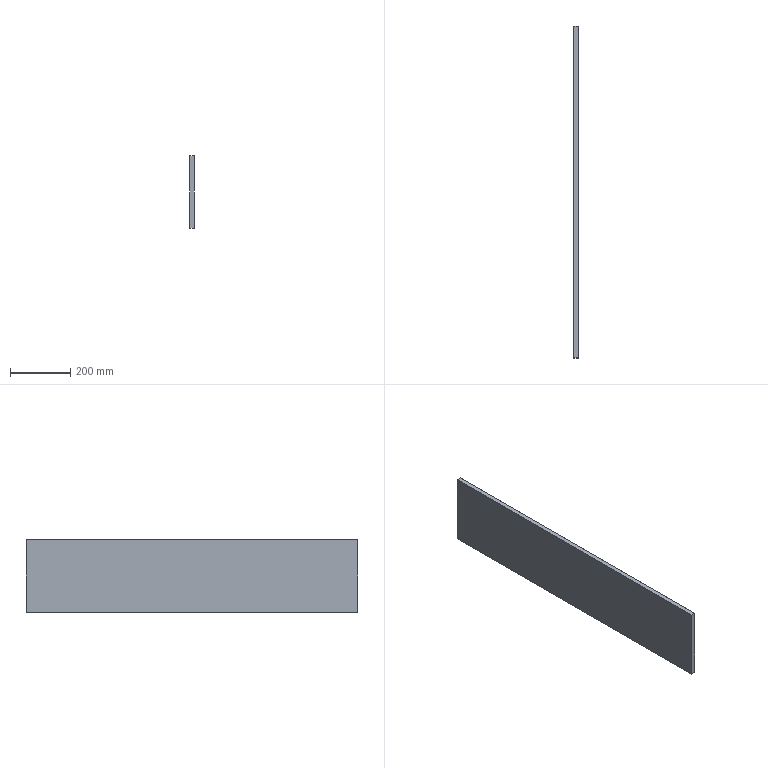Part | STEP file | HJDX-203 | 1 solid | 26 faces | box 16 x 1100 x 240 mm | volume 4223323 mm3 | plane 26
STEP:
#1=CARTESIAN_POINT('',(16.,-549.5,-119.5));
#2=VERTEX_POINT('',#1);
#3=CARTESIAN_POINT('',(16.,-549.5,119.5));
#4=VERTEX_POINT('',#3);
#5=CARTESIAN_POINT('',(16.,-549.5,0.));
#6=DIRECTION('',(0.,0.,1.));
#7=VECTOR('',#6,1000.);
#8=LINE('',#5,#7);
#9=EDGE_CURVE('',#2,#4,#8,.T.);
#10=ORIENTED_EDGE('',*,*,#9,.F.);
#11=CARTESIAN_POINT('',(16.,549.5,-119.5));
#12=VERTEX_POINT('',#11);
#13=CARTESIAN_POINT('',(16.,0.,-119.5));
#14=DIRECTION('',(0.,-1.,0.));
#15=VECTOR('',#14,1000.);
#16=LINE('',#13,#15);
#17=EDGE_CURVE('',#12,#2,#16,.T.);
#18=ORIENTED_EDGE('',*,*,#17,.F.);
#19=CARTESIAN_POINT('',(16.,549.5,119.5));
#20=VERTEX_POINT('',#19);
#21=CARTESIAN_POINT('',(16.,549.5,0.));
#22=DIRECTION('',(0.,0.,-1.));
#23=VECTOR('',#22,1000.);
#24=LINE('',#21,#23);
#25=EDGE_CURVE('',#20,#12,#24,.T.);
#26=ORIENTED_EDGE('',*,*,#25,.F.);
#27=CARTESIAN_POINT('',(16.,0.,119.5));
#28=DIRECTION('',(0.,1.,0.));
#29=VECTOR('',#28,1000.);
#30=LINE('',#27,#29);
#31=EDGE_CURVE('',#4,#20,#30,.T.);
#32=ORIENTED_EDGE('',*,*,#31,.F.);
#33=EDGE_LOOP('',(#10,#18,#26,#32));
#34=FACE_OUTER_BOUND('',#33,.T.);
#35=CARTESIAN_POINT('',(16.,0.,0.));
#36=DIRECTION('',(-1.,0.,0.));
#37=DIRECTION('',(0.,0.,1.));
#38=AXIS2_PLACEMENT_3D('',#35,#36,#37);
#39=PLANE('',#38);
#40=ADVANCED_FACE('',(#34),#39,.F.);
#41=CARTESIAN_POINT('',(15.5,-549.5,120.));
#42=VERTEX_POINT('',#41);
#43=CARTESIAN_POINT('',(15.5,549.5,120.));
#44=VERTEX_POINT('',#43);
#45=CARTESIAN_POINT('',(15.5,0.,120.));
#46=DIRECTION('',(0.,1.,0.));
#47=VECTOR('',#46,1000.);
#48=LINE('',#45,#47);
#49=EDGE_CURVE('',#42,#44,#48,.T.);
#50=ORIENTED_EDGE('',*,*,#49,.F.);
#51=CARTESIAN_POINT('',(16.,-549.5,119.5));
#52=DIRECTION('',(-0.7071,0.,0.7071));
#53=VECTOR('',#52,1000.);
#54=LINE('',#51,#53);
#55=EDGE_CURVE('',#4,#42,#54,.T.);
#56=ORIENTED_EDGE('',*,*,#55,.F.);
#57=ORIENTED_EDGE('',*,*,#31,.T.);
#58=CARTESIAN_POINT('',(16.,549.5,119.5));
#59=DIRECTION('',(0.7071,0.,-0.7071));
#60=VECTOR('',#59,1000.);
#61=LINE('',#58,#60);
#62=EDGE_CURVE('',#44,#20,#61,.T.);
#63=ORIENTED_EDGE('',*,*,#62,.F.);
#64=EDGE_LOOP('',(#50,#56,#57,#63));
#65=FACE_OUTER_BOUND('',#64,.T.);
#66=CARTESIAN_POINT('',(16.,0.,119.5));
#67=DIRECTION('',(-0.7071,0.,-0.7071));
#68=DIRECTION('',(-0.7071,0.,0.7071));
#69=AXIS2_PLACEMENT_3D('',#66,#67,#68);
#70=PLANE('',#69);
#71=ADVANCED_FACE('',(#65),#70,.F.);
#72=CARTESIAN_POINT('',(15.5,-550.,-119.5));
#73=VERTEX_POINT('',#72);
#74=CARTESIAN_POINT('',(15.5,-550.,119.5));
#75=VERTEX_POINT('',#74);
#76=CARTESIAN_POINT('',(15.5,-550.,0.));
#77=DIRECTION('',(0.,0.,1.));
#78=VECTOR('',#77,1000.);
#79=LINE('',#76,#78);
#80=EDGE_CURVE('',#73,#75,#79,.T.);
#81=ORIENTED_EDGE('',*,*,#80,.F.);
#82=CARTESIAN_POINT('',(16.,-549.5,-119.5));
#83=DIRECTION('',(-0.7071,-0.7071,0.));
#84=VECTOR('',#83,1000.);
#85=LINE('',#82,#84);
#86=EDGE_CURVE('',#2,#73,#85,.T.);
#87=ORIENTED_EDGE('',*,*,#86,.F.);
#88=ORIENTED_EDGE('',*,*,#9,.T.);
#89=CARTESIAN_POINT('',(16.,-549.5,119.5));
#90=DIRECTION('',(0.7071,0.7071,0.));
#91=VECTOR('',#90,1000.);
#92=LINE('',#89,#91);
#93=EDGE_CURVE('',#75,#4,#92,.T.);
#94=ORIENTED_EDGE('',*,*,#93,.F.);
#95=EDGE_LOOP('',(#81,#87,#88,#94));
#96=FACE_OUTER_BOUND('',#95,.T.);
#97=CARTESIAN_POINT('',(16.,-549.5,0.));
#98=DIRECTION('',(-0.7071,0.7071,0.));
#99=DIRECTION('',(-0.7071,-0.7071,0.));
#100=AXIS2_PLACEMENT_3D('',#97,#98,#99);
#101=PLANE('',#100);
#102=ADVANCED_FACE('',(#96),#101,.F.);
#103=ORIENTED_EDGE('',*,*,#17,.T.);
#104=CARTESIAN_POINT('',(15.5,-549.5,-120.));
#105=VERTEX_POINT('',#104);
#106=CARTESIAN_POINT('',(16.,-549.5,-119.5));
#107=DIRECTION('',(0.7071,0.,0.7071));
#108=VECTOR('',#107,1000.);
#109=LINE('',#106,#108);
#110=EDGE_CURVE('',#105,#2,#109,.T.);
#111=ORIENTED_EDGE('',*,*,#110,.F.);
#112=CARTESIAN_POINT('',(15.5,549.5,-120.));
#113=VERTEX_POINT('',#112);
#114=CARTESIAN_POINT('',(15.5,0.,-120.));
#115=DIRECTION('',(0.,-1.,0.));
#116=VECTOR('',#115,1000.);
#117=LINE('',#114,#116);
#118=EDGE_CURVE('',#113,#105,#117,.T.);
#119=ORIENTED_EDGE('',*,*,#118,.F.);
#120=CARTESIAN_POINT('',(16.,549.5,-119.5));
#121=DIRECTION('',(-0.7071,0.,-0.7071));
#122=VECTOR('',#121,1000.);
#123=LINE('',#120,#122);
#124=EDGE_CURVE('',#12,#113,#123,.T.);
#125=ORIENTED_EDGE('',*,*,#124,.F.);
#126=EDGE_LOOP('',(#103,#111,#119,#125));
#127=FACE_OUTER_BOUND('',#126,.T.);
#128=CARTESIAN_POINT('',(16.,0.,-119.5));
#129=DIRECTION('',(-0.7071,0.,0.7071));
#130=DIRECTION('',(0.7071,0.,0.7071));
#131=AXIS2_PLACEMENT_3D('',#128,#129,#130);
#132=PLANE('',#131);
#133=ADVANCED_FACE('',(#127),#132,.F.);
#134=ORIENTED_EDGE('',*,*,#25,.T.);
#135=CARTESIAN_POINT('',(15.5,550.,-119.5));
#136=VERTEX_POINT('',#135);
#137=CARTESIAN_POINT('',(16.,549.5,-119.5));
#138=DIRECTION('',(0.7071,-0.7071,0.));
#139=VECTOR('',#138,1000.);
#140=LINE('',#137,#139);
#141=EDGE_CURVE('',#136,#12,#140,.T.);
#142=ORIENTED_EDGE('',*,*,#141,.F.);
#143=CARTESIAN_POINT('',(15.5,550.,119.5));
#144=VERTEX_POINT('',#143);
#145=CARTESIAN_POINT('',(15.5,550.,0.));
#146=DIRECTION('',(0.,0.,-1.));
#147=VECTOR('',#146,1000.);
#148=LINE('',#145,#147);
#149=EDGE_CURVE('',#144,#136,#148,.T.);
#150=ORIENTED_EDGE('',*,*,#149,.F.);
#151=CARTESIAN_POINT('',(16.,549.5,119.5));
#152=DIRECTION('',(-0.7071,0.7071,0.));
#153=VECTOR('',#152,1000.);
#154=LINE('',#151,#153);
#155=EDGE_CURVE('',#20,#144,#154,.T.);
#156=ORIENTED_EDGE('',*,*,#155,.F.);
#157=EDGE_LOOP('',(#134,#142,#150,#156));
#158=FACE_OUTER_BOUND('',#157,.T.);
#159=CARTESIAN_POINT('',(16.,549.5,0.));
#160=DIRECTION('',(-0.7071,-0.7071,0.));
#161=DIRECTION('',(0.7071,-0.7071,0.));
#162=AXIS2_PLACEMENT_3D('',#159,#160,#161);
#163=PLANE('',#162);
#164=ADVANCED_FACE('',(#158),#163,.F.);
#165=CARTESIAN_POINT('',(15.5,549.5,120.));
#166=DIRECTION('',(0.,-0.7071,0.7071));
#167=VECTOR('',#166,1000.);
#168=LINE('',#165,#167);
#169=EDGE_CURVE('',#144,#44,#168,.T.);
#170=ORIENTED_EDGE('',*,*,#169,.T.);
#171=ORIENTED_EDGE('',*,*,#62,.T.);
#172=ORIENTED_EDGE('',*,*,#155,.T.);
#173=EDGE_LOOP('',(#170,#171,#172));
#174=FACE_OUTER_BOUND('',#173,.T.);
#175=CARTESIAN_POINT('',(15.5,550.,119.5));
#176=DIRECTION('',(0.5774,0.5774,0.5774));
#177=DIRECTION('',(0.7071,0.,-0.7071));
#178=AXIS2_PLACEMENT_3D('',#175,#176,#177);
#179=PLANE('',#178);
#180=ADVANCED_FACE('',(#174),#179,.T.);
#181=CARTESIAN_POINT('',(0.5,549.5,120.));
#182=VERTEX_POINT('',#181);
#183=CARTESIAN_POINT('',(16.,549.5,120.));
#184=DIRECTION('',(1.,0.,0.));
#185=VECTOR('',#184,1000.);
#186=LINE('',#183,#185);
#187=EDGE_CURVE('',#182,#44,#186,.T.);
#188=ORIENTED_EDGE('',*,*,#187,.F.);
#189=CARTESIAN_POINT('',(0.5,-549.5,120.));
#190=VERTEX_POINT('',#189);
#191=CARTESIAN_POINT('',(0.5,-550.,120.));
#192=DIRECTION('',(0.,1.,0.));
#193=VECTOR('',#192,1000.);
#194=LINE('',#191,#193);
#195=EDGE_CURVE('',#190,#182,#194,.T.);
#196=ORIENTED_EDGE('',*,*,#195,.F.);
#197=CARTESIAN_POINT('',(16.,-549.5,120.));
#198=DIRECTION('',(-1.,0.,0.));
#199=VECTOR('',#198,1000.);
#200=LINE('',#197,#199);
#201=EDGE_CURVE('',#42,#190,#200,.T.);
#202=ORIENTED_EDGE('',*,*,#201,.F.);
#203=ORIENTED_EDGE('',*,*,#49,.T.);
#204=EDGE_LOOP('',(#188,#196,#202,#203));
#205=FACE_OUTER_BOUND('',#204,.T.);
#206=CARTESIAN_POINT('',(16.,-550.,120.));
#207=DIRECTION('',(0.,0.,-1.));
#208=DIRECTION('',(-1.,0.,0.));
#209=AXIS2_PLACEMENT_3D('',#206,#207,#208);
#210=PLANE('',#209);
#211=ADVANCED_FACE('',(#205),#210,.F.);
#212=CARTESIAN_POINT('',(15.5,-549.5,120.));
#213=DIRECTION('',(0.,-0.7071,-0.7071));
#214=VECTOR('',#213,1000.);
#215=LINE('',#212,#214);
#216=EDGE_CURVE('',#42,#75,#215,.T.);
#217=ORIENTED_EDGE('',*,*,#216,.T.);
#218=ORIENTED_EDGE('',*,*,#93,.T.);
#219=ORIENTED_EDGE('',*,*,#55,.T.);
#220=EDGE_LOOP('',(#217,#218,#219));
#221=FACE_OUTER_BOUND('',#220,.T.);
#222=CARTESIAN_POINT('',(15.5,-549.5,120.));
#223=DIRECTION('',(0.5774,-0.5774,0.5774));
#224=DIRECTION('',(0.7071,0.,-0.7071));
#225=AXIS2_PLACEMENT_3D('',#222,#223,#224);
#226=PLANE('',#225);
#227=ADVANCED_FACE('',(#221),#226,.T.);
#228=CARTESIAN_POINT('',(0.5,-550.,-119.5));
#229=VERTEX_POINT('',#228);
#230=CARTESIAN_POINT('',(16.,-550.,-119.5));
#231=DIRECTION('',(-1.,0.,0.));
#232=VECTOR('',#231,1000.);
#233=LINE('',#230,#232);
#234=EDGE_CURVE('',#73,#229,#233,.T.);
#235=ORIENTED_EDGE('',*,*,#234,.F.);
#236=ORIENTED_EDGE('',*,*,#80,.T.);
#237=CARTESIAN_POINT('',(0.5,-550.,119.5));
#238=VERTEX_POINT('',#237);
#239=CARTESIAN_POINT('',(16.,-550.,119.5));
#240=DIRECTION('',(1.,0.,0.));
#241=VECTOR('',#240,1000.);
#242=LINE('',#239,#241);
#243=EDGE_CURVE('',#238,#75,#242,.T.);
#244=ORIENTED_EDGE('',*,*,#243,.F.);
#245=CARTESIAN_POINT('',(0.5,-550.,120.));
#246=DIRECTION('',(0.,0.,1.));
#247=VECTOR('',#246,1000.);
#248=LINE('',#245,#247);
#249=EDGE_CURVE('',#229,#238,#248,.T.);
#250=ORIENTED_EDGE('',*,*,#249,.F.);
#251=EDGE_LOOP('',(#235,#236,#244,#250));
#252=FACE_OUTER_BOUND('',#251,.T.);
#253=CARTESIAN_POINT('',(16.,-550.,120.));
#254=DIRECTION('',(0.,1.,0.));
#255=DIRECTION('',(0.,0.,1.));
#256=AXIS2_PLACEMENT_3D('',#253,#254,#255);
#257=PLANE('',#256);
#258=ADVANCED_FACE('',(#252),#257,.F.);
#259=ORIENTED_EDGE('',*,*,#86,.T.);
#260=CARTESIAN_POINT('',(15.5,-550.,-119.5));
#261=DIRECTION('',(0.,0.7071,-0.7071));
#262=VECTOR('',#261,1000.);
#263=LINE('',#260,#262);
#264=EDGE_CURVE('',#73,#105,#263,.T.);
#265=ORIENTED_EDGE('',*,*,#264,.T.);
#266=ORIENTED_EDGE('',*,*,#110,.T.);
#267=EDGE_LOOP('',(#259,#265,#266));
#268=FACE_OUTER_BOUND('',#267,.T.);
#269=CARTESIAN_POINT('',(15.5,-550.,-119.5));
#270=DIRECTION('',(0.5774,-0.5774,-0.5774));
#271=DIRECTION('',(-0.7071,0.,-0.7071));
#272=AXIS2_PLACEMENT_3D('',#269,#270,#271);
#273=PLANE('',#272);
#274=ADVANCED_FACE('',(#268),#273,.T.);
#275=ORIENTED_EDGE('',*,*,#141,.T.);
#276=ORIENTED_EDGE('',*,*,#124,.T.);
#277=CARTESIAN_POINT('',(15.5,550.,-119.5));
#278=DIRECTION('',(0.,0.7071,0.7071));
#279=VECTOR('',#278,1000.);
#280=LINE('',#277,#279);
#281=EDGE_CURVE('',#113,#136,#280,.T.);
#282=ORIENTED_EDGE('',*,*,#281,.T.);
#283=EDGE_LOOP('',(#275,#276,#282));
#284=FACE_OUTER_BOUND('',#283,.T.);
#285=CARTESIAN_POINT('',(15.5,549.5,-120.));
#286=DIRECTION('',(0.5774,0.5774,-0.5774));
#287=DIRECTION('',(-0.7071,0.,-0.7071));
#288=AXIS2_PLACEMENT_3D('',#285,#286,#287);
#289=PLANE('',#288);
#290=ADVANCED_FACE('',(#284),#289,.T.);
#291=CARTESIAN_POINT('',(0.5,549.5,-120.));
#292=VERTEX_POINT('',#291);
#293=CARTESIAN_POINT('',(0.5,-549.5,-120.));
#294=VERTEX_POINT('',#293);
#295=CARTESIAN_POINT('',(0.5,-550.,-120.));
#296=DIRECTION('',(0.,-1.,0.));
#297=VECTOR('',#296,1000.);
#298=LINE('',#295,#297);
#299=EDGE_CURVE('',#292,#294,#298,.T.);
#300=ORIENTED_EDGE('',*,*,#299,.F.);
#301=CARTESIAN_POINT('',(16.,549.5,-120.));
#302=DIRECTION('',(-1.,0.,0.));
#303=VECTOR('',#302,1000.);
#304=LINE('',#301,#303);
#305=EDGE_CURVE('',#113,#292,#304,.T.);
#306=ORIENTED_EDGE('',*,*,#305,.F.);
#307=ORIENTED_EDGE('',*,*,#118,.T.);
#308=CARTESIAN_POINT('',(16.,-549.5,-120.));
#309=DIRECTION('',(1.,0.,0.));
#310=VECTOR('',#309,1000.);
#311=LINE('',#308,#310);
#312=EDGE_CURVE('',#294,#105,#311,.T.);
#313=ORIENTED_EDGE('',*,*,#312,.F.);
#314=EDGE_LOOP('',(#300,#306,#307,#313));
#315=FACE_OUTER_BOUND('',#314,.T.);
#316=CARTESIAN_POINT('',(16.,-550.,-120.));
#317=DIRECTION('',(0.,0.,1.));
#318=DIRECTION('',(1.,0.,0.));
#319=AXIS2_PLACEMENT_3D('',#316,#317,#318);
#320=PLANE('',#319);
#321=ADVANCED_FACE('',(#315),#320,.F.);
#322=CARTESIAN_POINT('',(0.5,550.,119.5));
#323=VERTEX_POINT('',#322);
#324=CARTESIAN_POINT('',(0.5,550.,-119.5));
#325=VERTEX_POINT('',#324);
#326=CARTESIAN_POINT('',(0.5,550.,120.));
#327=DIRECTION('',(0.,0.,-1.));
#328=VECTOR('',#327,1000.);
#329=LINE('',#326,#328);
#330=EDGE_CURVE('',#323,#325,#329,.T.);
#331=ORIENTED_EDGE('',*,*,#330,.F.);
#332=CARTESIAN_POINT('',(16.,550.,119.5));
#333=DIRECTION('',(-1.,0.,0.));
#334=VECTOR('',#333,1000.);
#335=LINE('',#332,#334);
#336=EDGE_CURVE('',#144,#323,#335,.T.);
#337=ORIENTED_EDGE('',*,*,#336,.F.);
#338=ORIENTED_EDGE('',*,*,#149,.T.);
#339=CARTESIAN_POINT('',(16.,550.,-119.5));
#340=DIRECTION('',(1.,0.,0.));
#341=VECTOR('',#340,1000.);
#342=LINE('',#339,#341);
#343=EDGE_CURVE('',#325,#136,#342,.T.);
#344=ORIENTED_EDGE('',*,*,#343,.F.);
#345=EDGE_LOOP('',(#331,#337,#338,#344));
#346=FACE_OUTER_BOUND('',#345,.T.);
#347=CARTESIAN_POINT('',(16.,550.,120.));
#348=DIRECTION('',(0.,-1.,0.));
#349=DIRECTION('',(0.,0.,-1.));
#350=AXIS2_PLACEMENT_3D('',#347,#348,#349);
#351=PLANE('',#350);
#352=ADVANCED_FACE('',(#346),#351,.F.);
#353=ORIENTED_EDGE('',*,*,#336,.T.);
#354=CARTESIAN_POINT('',(0.5,549.5,120.));
#355=DIRECTION('',(0.,0.7071,-0.7071));
#356=VECTOR('',#355,1000.);
#357=LINE('',#354,#356);
#358=EDGE_CURVE('',#182,#323,#357,.T.);
#359=ORIENTED_EDGE('',*,*,#358,.F.);
#360=ORIENTED_EDGE('',*,*,#187,.T.);
#361=ORIENTED_EDGE('',*,*,#169,.F.);
#362=EDGE_LOOP('',(#353,#359,#360,#361));
#363=FACE_OUTER_BOUND('',#362,.T.);
#364=CARTESIAN_POINT('',(16.,549.5,120.));
#365=DIRECTION('',(0.,-0.7071,-0.7071));
#366=DIRECTION('',(0.,0.7071,-0.7071));
#367=AXIS2_PLACEMENT_3D('',#364,#365,#366);
#368=PLANE('',#367);
#369=ADVANCED_FACE('',(#363),#368,.F.);
#370=CARTESIAN_POINT('',(0.,-549.5,119.5));
#371=VERTEX_POINT('',#370);
#372=CARTESIAN_POINT('',(0.5,-549.5,120.));
#373=DIRECTION('',(0.7071,0.,0.7071));
#374=VECTOR('',#373,1000.);
#375=LINE('',#372,#374);
#376=EDGE_CURVE('',#371,#190,#375,.T.);
#377=ORIENTED_EDGE('',*,*,#376,.T.);
#378=ORIENTED_EDGE('',*,*,#195,.T.);
#379=CARTESIAN_POINT('',(0.,549.5,119.5));
#380=VERTEX_POINT('',#379);
#381=CARTESIAN_POINT('',(0.5,549.5,120.));
#382=DIRECTION('',(-0.7071,0.,-0.7071));
#383=VECTOR('',#382,1000.);
#384=LINE('',#381,#383);
#385=EDGE_CURVE('',#182,#380,#384,.T.);
#386=ORIENTED_EDGE('',*,*,#385,.T.);
#387=CARTESIAN_POINT('',(0.,-550.,119.5));
#388=DIRECTION('',(0.,-1.,0.));
#389=VECTOR('',#388,1000.);
#390=LINE('',#387,#389);
#391=EDGE_CURVE('',#380,#371,#390,.T.);
#392=ORIENTED_EDGE('',*,*,#391,.T.);
#393=EDGE_LOOP('',(#377,#378,#386,#392));
#394=FACE_OUTER_BOUND('',#393,.T.);
#395=CARTESIAN_POINT('',(0.5,-550.,120.));
#396=DIRECTION('',(-0.7071,0.,0.7071));
#397=DIRECTION('',(0.7071,0.,0.7071));
#398=AXIS2_PLACEMENT_3D('',#395,#396,#397);
#399=PLANE('',#398);
#400=ADVANCED_FACE('',(#394),#399,.T.);
#401=ORIENTED_EDGE('',*,*,#201,.T.);
#402=CARTESIAN_POINT('',(0.5,-550.,119.5));
#403=DIRECTION('',(0.,0.7071,0.7071));
#404=VECTOR('',#403,1000.);
#405=LINE('',#402,#404);
#406=EDGE_CURVE('',#238,#190,#405,.T.);
#407=ORIENTED_EDGE('',*,*,#406,.F.);
#408=ORIENTED_EDGE('',*,*,#243,.T.);
#409=ORIENTED_EDGE('',*,*,#216,.F.);
#410=EDGE_LOOP('',(#401,#407,#408,#409));
#411=FACE_OUTER_BOUND('',#410,.T.);
#412=CARTESIAN_POINT('',(16.,-550.,119.5));
#413=DIRECTION('',(0.,0.7071,-0.7071));
#414=DIRECTION('',(0.,0.7071,0.7071));
#415=AXIS2_PLACEMENT_3D('',#412,#413,#414);
#416=PLANE('',#415);
#417=ADVANCED_FACE('',(#411),#416,.F.);
#418=CARTESIAN_POINT('',(0.,-549.5,-119.5));
#419=VERTEX_POINT('',#418);
#420=CARTESIAN_POINT('',(0.5,-550.,-119.5));
#421=DIRECTION('',(0.7071,-0.7071,0.));
#422=VECTOR('',#421,1000.);
#423=LINE('',#420,#422);
#424=EDGE_CURVE('',#419,#229,#423,.T.);
#425=ORIENTED_EDGE('',*,*,#424,.T.);
#426=ORIENTED_EDGE('',*,*,#249,.T.);
#427=CARTESIAN_POINT('',(0.5,-550.,119.5));
#428=DIRECTION('',(-0.7071,0.7071,0.));
#429=VECTOR('',#428,1000.);
#430=LINE('',#427,#429);
#431=EDGE_CURVE('',#238,#371,#430,.T.);
#432=ORIENTED_EDGE('',*,*,#431,.T.);
#433=CARTESIAN_POINT('',(0.,-549.5,120.));
#434=DIRECTION('',(0.,0.,-1.));
#435=VECTOR('',#434,1000.);
#436=LINE('',#433,#435);
#437=EDGE_CURVE('',#371,#419,#436,.T.);
#438=ORIENTED_EDGE('',*,*,#437,.T.);
#439=EDGE_LOOP('',(#425,#426,#432,#438));
#440=FACE_OUTER_BOUND('',#439,.T.);
#441=CARTESIAN_POINT('',(0.5,-550.,120.));
#442=DIRECTION('',(-0.7071,-0.7071,0.));
#443=DIRECTION('',(0.7071,-0.7071,0.));
#444=AXIS2_PLACEMENT_3D('',#441,#442,#443);
#445=PLANE('',#444);
#446=ADVANCED_FACE('',(#440),#445,.T.);
#447=ORIENTED_EDGE('',*,*,#234,.T.);
#448=CARTESIAN_POINT('',(0.5,-549.5,-120.));
#449=DIRECTION('',(0.,-0.7071,0.7071));
#450=VECTOR('',#449,1000.);
#451=LINE('',#448,#450);
#452=EDGE_CURVE('',#294,#229,#451,.T.);
#453=ORIENTED_EDGE('',*,*,#452,.F.);
#454=ORIENTED_EDGE('',*,*,#312,.T.);
#455=ORIENTED_EDGE('',*,*,#264,.F.);
#456=EDGE_LOOP('',(#447,#453,#454,#455));
#457=FACE_OUTER_BOUND('',#456,.T.);
#458=CARTESIAN_POINT('',(16.,-549.5,-120.));
#459=DIRECTION('',(0.,0.7071,0.7071));
#460=DIRECTION('',(0.,-0.7071,0.7071));
#461=AXIS2_PLACEMENT_3D('',#458,#459,#460);
#462=PLANE('',#461);
#463=ADVANCED_FACE('',(#457),#462,.F.);
#464=CARTESIAN_POINT('',(0.5,-549.5,-120.));
#465=DIRECTION('',(-0.7071,0.,0.7071));
#466=VECTOR('',#465,1000.);
#467=LINE('',#464,#466);
#468=EDGE_CURVE('',#294,#419,#467,.T.);
#469=ORIENTED_EDGE('',*,*,#468,.T.);
#470=CARTESIAN_POINT('',(0.,549.5,-119.5));
#471=VERTEX_POINT('',#470);
#472=CARTESIAN_POINT('',(0.,-550.,-119.5));
#473=DIRECTION('',(0.,1.,0.));
#474=VECTOR('',#473,1000.);
#475=LINE('',#472,#474);
#476=EDGE_CURVE('',#419,#471,#475,.T.);
#477=ORIENTED_EDGE('',*,*,#476,.T.);
#478=CARTESIAN_POINT('',(0.5,549.5,-120.));
#479=DIRECTION('',(0.7071,0.,-0.7071));
#480=VECTOR('',#479,1000.);
#481=LINE('',#478,#480);
#482=EDGE_CURVE('',#471,#292,#481,.T.);
#483=ORIENTED_EDGE('',*,*,#482,.T.);
#484=ORIENTED_EDGE('',*,*,#299,.T.);
#485=EDGE_LOOP('',(#469,#477,#483,#484));
#486=FACE_OUTER_BOUND('',#485,.T.);
#487=CARTESIAN_POINT('',(0.5,-550.,-120.));
#488=DIRECTION('',(-0.7071,0.,-0.7071));
#489=DIRECTION('',(-0.7071,0.,0.7071));
#490=AXIS2_PLACEMENT_3D('',#487,#488,#489);
#491=PLANE('',#490);
#492=ADVANCED_FACE('',(#486),#491,.T.);
#493=ORIENTED_EDGE('',*,*,#343,.T.);
#494=ORIENTED_EDGE('',*,*,#281,.F.);
#495=ORIENTED_EDGE('',*,*,#305,.T.);
#496=CARTESIAN_POINT('',(0.5,550.,-119.5));
#497=DIRECTION('',(0.,-0.7071,-0.7071));
#498=VECTOR('',#497,1000.);
#499=LINE('',#496,#498);
#500=EDGE_CURVE('',#325,#292,#499,.T.);
#501=ORIENTED_EDGE('',*,*,#500,.F.);
#502=EDGE_LOOP('',(#493,#494,#495,#501));
#503=FACE_OUTER_BOUND('',#502,.T.);
#504=CARTESIAN_POINT('',(16.,550.,-119.5));
#505=DIRECTION('',(0.,-0.7071,0.7071));
#506=DIRECTION('',(0.,-0.7071,-0.7071));
#507=AXIS2_PLACEMENT_3D('',#504,#505,#506);
#508=PLANE('',#507);
#509=ADVANCED_FACE('',(#503),#508,.F.);
#510=CARTESIAN_POINT('',(0.5,550.,-119.5));
#511=DIRECTION('',(-0.7071,-0.7071,0.));
#512=VECTOR('',#511,1000.);
#513=LINE('',#510,#512);
#514=EDGE_CURVE('',#325,#471,#513,.T.);
#515=ORIENTED_EDGE('',*,*,#514,.T.);
#516=CARTESIAN_POINT('',(0.,549.5,120.));
#517=DIRECTION('',(0.,0.,1.));
#518=VECTOR('',#517,1000.);
#519=LINE('',#516,#518);
#520=EDGE_CURVE('',#471,#380,#519,.T.);
#521=ORIENTED_EDGE('',*,*,#520,.T.);
#522=CARTESIAN_POINT('',(0.5,550.,119.5));
#523=DIRECTION('',(0.7071,0.7071,0.));
#524=VECTOR('',#523,1000.);
#525=LINE('',#522,#524);
#526=EDGE_CURVE('',#380,#323,#525,.T.);
#527=ORIENTED_EDGE('',*,*,#526,.T.);
#528=ORIENTED_EDGE('',*,*,#330,.T.);
#529=EDGE_LOOP('',(#515,#521,#527,#528));
#530=FACE_OUTER_BOUND('',#529,.T.);
#531=CARTESIAN_POINT('',(0.5,550.,120.));
#532=DIRECTION('',(-0.7071,0.7071,0.));
#533=DIRECTION('',(-0.7071,-0.7071,0.));
#534=AXIS2_PLACEMENT_3D('',#531,#532,#533);
#535=PLANE('',#534);
#536=ADVANCED_FACE('',(#530),#535,.T.);
#537=ORIENTED_EDGE('',*,*,#358,.T.);
#538=ORIENTED_EDGE('',*,*,#526,.F.);
#539=ORIENTED_EDGE('',*,*,#385,.F.);
#540=EDGE_LOOP('',(#537,#538,#539));
#541=FACE_OUTER_BOUND('',#540,.T.);
#542=CARTESIAN_POINT('',(0.5,549.5,120.));
#543=DIRECTION('',(-0.5774,0.5774,0.5774));
#544=DIRECTION('',(0.7071,0.,0.7071));
#545=AXIS2_PLACEMENT_3D('',#542,#543,#544);
#546=PLANE('',#545);
#547=ADVANCED_FACE('',(#541),#546,.T.);
#548=ORIENTED_EDGE('',*,*,#376,.F.);
#549=ORIENTED_EDGE('',*,*,#431,.F.);
#550=ORIENTED_EDGE('',*,*,#406,.T.);
#551=EDGE_LOOP('',(#548,#549,#550));
#552=FACE_OUTER_BOUND('',#551,.T.);
#553=CARTESIAN_POINT('',(0.5,-549.5,120.));
#554=DIRECTION('',(-0.5774,-0.5774,0.5774));
#555=DIRECTION('',(0.7071,0.,0.7071));
#556=AXIS2_PLACEMENT_3D('',#553,#554,#555);
#557=PLANE('',#556);
#558=ADVANCED_FACE('',(#552),#557,.T.);
#559=ORIENTED_EDGE('',*,*,#476,.F.);
#560=ORIENTED_EDGE('',*,*,#437,.F.);
#561=ORIENTED_EDGE('',*,*,#391,.F.);
#562=ORIENTED_EDGE('',*,*,#520,.F.);
#563=EDGE_LOOP('',(#559,#560,#561,#562));
#564=FACE_OUTER_BOUND('',#563,.T.);
#565=CARTESIAN_POINT('',(0.,0.,0.));
#566=DIRECTION('',(-1.,0.,0.));
#567=DIRECTION('',(0.,0.,1.));
#568=AXIS2_PLACEMENT_3D('',#565,#566,#567);
#569=PLANE('',#568);
#570=ADVANCED_FACE('',(#564),#569,.T.);
#571=ORIENTED_EDGE('',*,*,#468,.F.);
#572=ORIENTED_EDGE('',*,*,#452,.T.);
#573=ORIENTED_EDGE('',*,*,#424,.F.);
#574=EDGE_LOOP('',(#571,#572,#573));
#575=FACE_OUTER_BOUND('',#574,.T.);
#576=CARTESIAN_POINT('',(0.5,-549.5,-120.));
#577=DIRECTION('',(-0.5774,-0.5774,-0.5774));
#578=DIRECTION('',(-0.7071,0.,0.7071));
#579=AXIS2_PLACEMENT_3D('',#576,#577,#578);
#580=PLANE('',#579);
#581=ADVANCED_FACE('',(#575),#580,.T.);
#582=ORIENTED_EDGE('',*,*,#500,.T.);
#583=ORIENTED_EDGE('',*,*,#482,.F.);
#584=ORIENTED_EDGE('',*,*,#514,.F.);
#585=EDGE_LOOP('',(#582,#583,#584));
#586=FACE_OUTER_BOUND('',#585,.T.);
#587=CARTESIAN_POINT('',(0.5,550.,-119.5));
#588=DIRECTION('',(-0.5774,0.5774,-0.5774));
#589=DIRECTION('',(-0.7071,0.,0.7071));
#590=AXIS2_PLACEMENT_3D('',#587,#588,#589);
#591=PLANE('',#590);
#592=ADVANCED_FACE('',(#586),#591,.T.);
#593=CLOSED_SHELL('',(#40,#71,#102,#133,#164,#180,#211,#227,#258,#274,#290,#321,#352,#369,#400,#417,#446,#463,#492,#509,#536,#547,#558,#570,#581,#592));
#594=MANIFOLD_SOLID_BREP('',#593);
#595=CARTESIAN_POINT('',(0.,0.,0.));
#596=DIRECTION('',(0.,0.,1.));
#597=DIRECTION('',(1.,0.,0.));
#598=AXIS2_PLACEMENT_3D('',#595,#596,#597);
#599=(LENGTH_UNIT()NAMED_UNIT(*)SI_UNIT(.MILLI.,.METRE.));
#600=UNCERTAINTY_MEASURE_WITH_UNIT(LENGTH_MEASURE(0.00001),#599,'','');
#601=(NAMED_UNIT(*)PLANE_ANGLE_UNIT()SI_UNIT($,.RADIAN.));
#602=(NAMED_UNIT(*)SI_UNIT($,.STERADIAN.)SOLID_ANGLE_UNIT());
#603=(GEOMETRIC_REPRESENTATION_CONTEXT(3)GLOBAL_UNCERTAINTY_ASSIGNED_CONTEXT((#600))GLOBAL_UNIT_ASSIGNED_CONTEXT((#599,#601,#602))REPRESENTATION_CONTEXT('',''));
#604=ADVANCED_BREP_SHAPE_REPRESENTATION('',(#594,#598),#603);